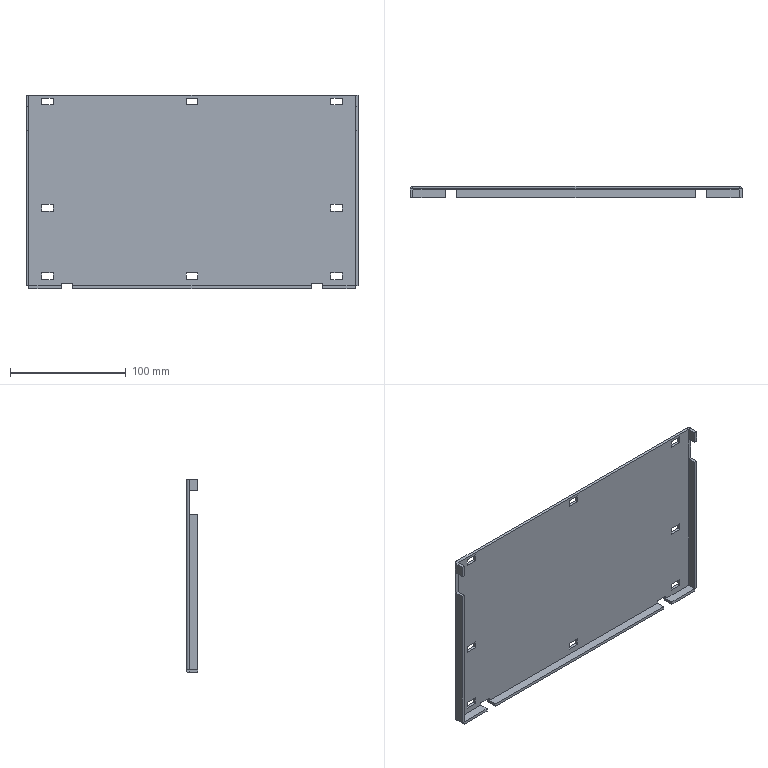Part | NX | features solid 2 | 1 solid | 93 faces | box 287 x 10 x 167.5 mm | volume 128218 mm3 | plane 88 | cylinder 5 | commonest cylinder face diameters 5 x5